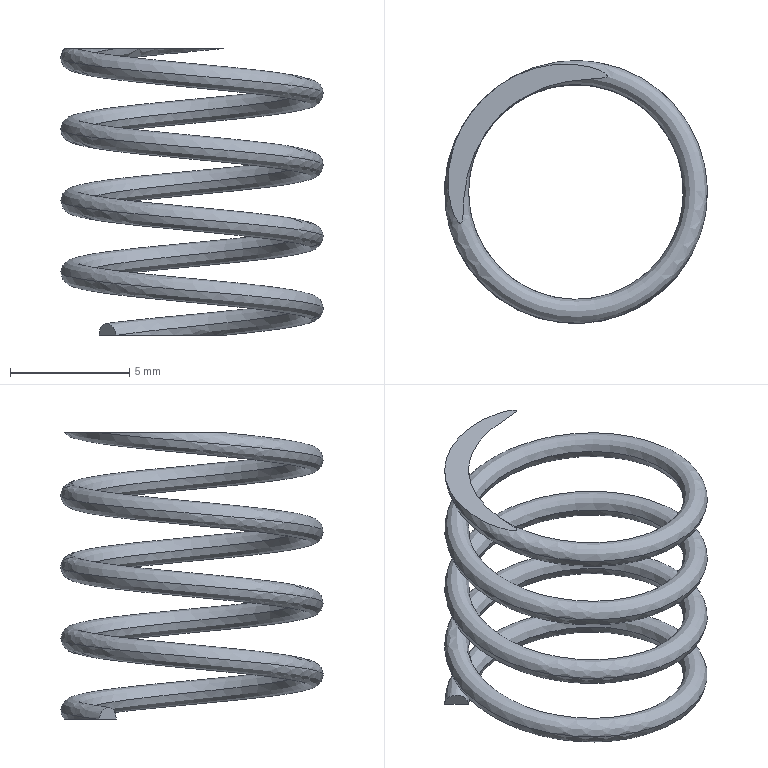Part | SolidWorks | features Helix 1, ICE 1, Sweep 1 | 1 solid | 5 faces | box 11 x 11 x 12 mm | volume 96.988 mm3 | plane 3 | spline 2